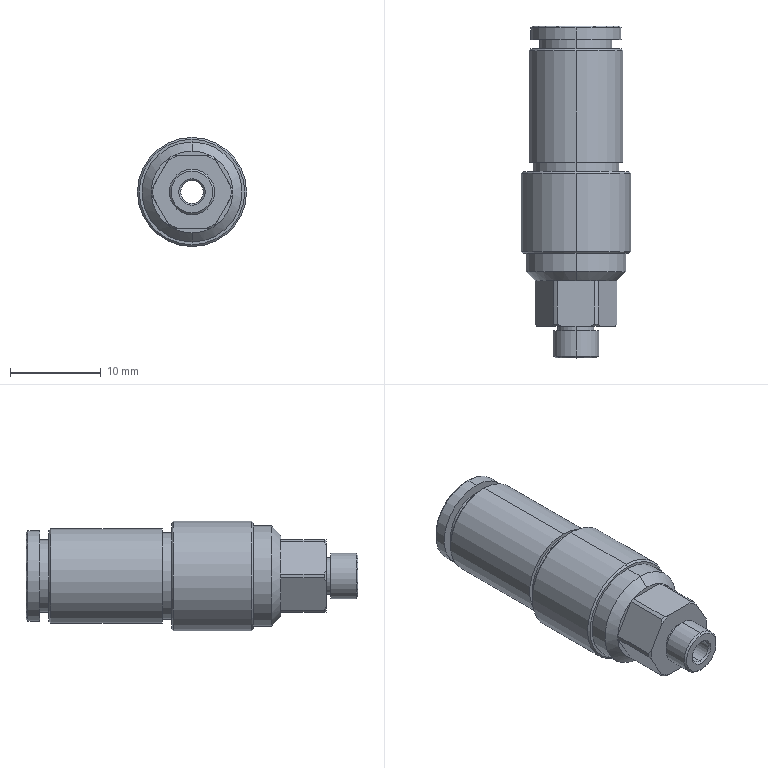Part | SolidWorks | features ICE 1, Revolution 1 | 1 solid | 71 faces | box 12 x 36.5 x 12 mm | volume 2508 mm3 | cylinder 26 | cone 24 | plane 21 | commonest cylinder face diameters 9 x6 4 x4 2.5 x2 5 x2 8 x2 9.5 x2